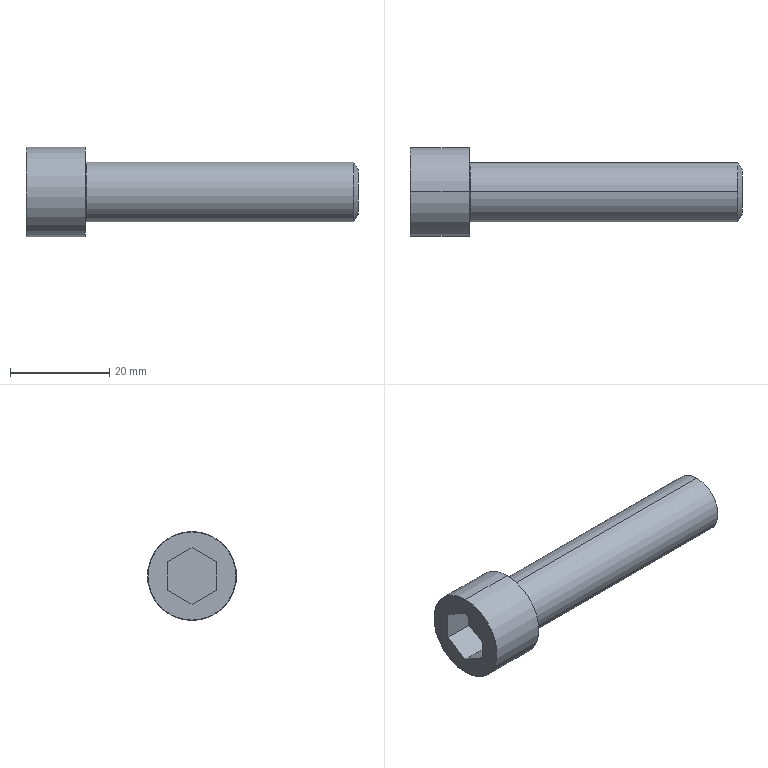Part | SolidWorks | features BaseBody 1 | 1 solid | 20 faces | box 67 x 18 x 18 mm | volume 8742 mm3 | plane 10 | torus 4 | cylinder 4 | cone 2 | commonest cylinder face diameters 12 x2 18 x2
STEP:
#1=CARTESIAN_POINT('',(0.,0.,8.9));
#2=VERTEX_POINT('',#1);
#3=CARTESIAN_POINT('',(0.1,0.,9.));
#4=VERTEX_POINT('',#3);
#5=CARTESIAN_POINT('',(0.1,0.,8.9));
#6=DIRECTION('',(0.,1.,0.));
#7=DIRECTION('',(0.,0.,1.));
#8=AXIS2_PLACEMENT_3D('',#5,#6,#7);
#9=CIRCLE('',#8,0.1);
#10=EDGE_CURVE('',#2,#4,#9,.T.);
#11=ORIENTED_EDGE('',*,*,#10,.F.);
#12=CARTESIAN_POINT('',(0.,0.,-8.9));
#13=VERTEX_POINT('',#12);
#14=CARTESIAN_POINT('',(0.,0.,0.));
#15=DIRECTION('',(-1.,0.,0.));
#16=DIRECTION('',(0.,0.,-1.));
#17=AXIS2_PLACEMENT_3D('',#14,#15,#16);
#18=CIRCLE('',#17,8.9);
#19=EDGE_CURVE('',#13,#2,#18,.T.);
#20=ORIENTED_EDGE('',*,*,#19,.F.);
#21=CARTESIAN_POINT('',(0.1,0.,-9.));
#22=VERTEX_POINT('',#21);
#23=CARTESIAN_POINT('',(0.1,0.,-8.9));
#24=DIRECTION('',(0.,-1.,0.));
#25=DIRECTION('',(0.,0.,-1.));
#26=AXIS2_PLACEMENT_3D('',#23,#24,#25);
#27=CIRCLE('',#26,0.1);
#28=EDGE_CURVE('',#13,#22,#27,.T.);
#29=ORIENTED_EDGE('',*,*,#28,.T.);
#30=CARTESIAN_POINT('',(0.1,0.,0.));
#31=DIRECTION('',(1.,0.,0.));
#32=DIRECTION('',(0.,0.,-1.));
#33=AXIS2_PLACEMENT_3D('',#30,#31,#32);
#34=CIRCLE('',#33,9.);
#35=EDGE_CURVE('',#4,#22,#34,.T.);
#36=ORIENTED_EDGE('',*,*,#35,.F.);
#37=EDGE_LOOP('',(#11,#20,#29,#36));
#38=FACE_OUTER_BOUND('',#37,.T.);
#39=CARTESIAN_POINT('',(0.1,0.,0.));
#40=DIRECTION('',(1.,0.,0.));
#41=DIRECTION('',(0.,0.,-1.));
#42=AXIS2_PLACEMENT_3D('',#39,#40,#41);
#43=TOROIDAL_SURFACE('',#42,8.9,0.1);
#44=ADVANCED_FACE('',(#38),#43,.T.);
#45=CARTESIAN_POINT('',(67.,0.,4.484));
#46=VERTEX_POINT('',#45);
#47=CARTESIAN_POINT('',(67.,0.,-4.484));
#48=VERTEX_POINT('',#47);
#49=CARTESIAN_POINT('',(67.,0.,0.));
#50=DIRECTION('',(-1.,0.,0.));
#51=DIRECTION('',(0.,0.,1.));
#52=AXIS2_PLACEMENT_3D('',#49,#50,#51);
#53=CIRCLE('',#52,4.484);
#54=EDGE_CURVE('',#46,#48,#53,.T.);
#55=ORIENTED_EDGE('',*,*,#54,.F.);
#56=CARTESIAN_POINT('',(67.,0.,0.));
#57=DIRECTION('',(-1.,0.,0.));
#58=DIRECTION('',(0.,0.,1.));
#59=AXIS2_PLACEMENT_3D('',#56,#57,#58);
#60=CIRCLE('',#59,4.484);
#61=EDGE_CURVE('',#48,#46,#60,.T.);
#62=ORIENTED_EDGE('',*,*,#61,.F.);
#63=EDGE_LOOP('',(#55,#62));
#64=FACE_OUTER_BOUND('',#63,.T.);
#65=CARTESIAN_POINT('',(67.,6.,0.));
#66=DIRECTION('',(-1.,0.,0.));
#67=DIRECTION('',(0.,0.,1.));
#68=AXIS2_PLACEMENT_3D('',#65,#66,#67);
#69=PLANE('',#68);
#70=ADVANCED_FACE('',(#64),#69,.F.);
#71=CARTESIAN_POINT('',(66.125,0.,-6.));
#72=VERTEX_POINT('',#71);
#73=CARTESIAN_POINT('',(66.125,0.,-6.));
#74=DIRECTION('',(-0.5,0.,-0.866));
#75=VECTOR('',#74,1000.);
#76=LINE('',#73,#75);
#77=EDGE_CURVE('',#48,#72,#76,.T.);
#78=ORIENTED_EDGE('',*,*,#77,.F.);
#79=ORIENTED_EDGE('',*,*,#61,.T.);
#80=CARTESIAN_POINT('',(66.125,0.,6.));
#81=VERTEX_POINT('',#80);
#82=CARTESIAN_POINT('',(66.125,0.,6.));
#83=DIRECTION('',(-0.5,0.,0.866));
#84=VECTOR('',#83,1000.);
#85=LINE('',#82,#84);
#86=EDGE_CURVE('',#46,#81,#85,.T.);
#87=ORIENTED_EDGE('',*,*,#86,.T.);
#88=CARTESIAN_POINT('',(66.125,0.,0.));
#89=DIRECTION('',(-1.,0.,0.));
#90=DIRECTION('',(0.,0.,1.));
#91=AXIS2_PLACEMENT_3D('',#88,#89,#90);
#92=CIRCLE('',#91,6.);
#93=EDGE_CURVE('',#72,#81,#92,.T.);
#94=ORIENTED_EDGE('',*,*,#93,.F.);
#95=EDGE_LOOP('',(#78,#79,#87,#94));
#96=FACE_OUTER_BOUND('',#95,.T.);
#97=CARTESIAN_POINT('',(66.125,0.,0.));
#98=DIRECTION('',(-1.,0.,0.));
#99=DIRECTION('',(0.,0.,1.));
#100=AXIS2_PLACEMENT_3D('',#97,#98,#99);
#101=CONICAL_SURFACE('',#100,6.,1.047);
#102=ADVANCED_FACE('',(#96),#101,.T.);
#103=CARTESIAN_POINT('',(6.,-4.949,2.857));
#104=VERTEX_POINT('',#103);
#105=CARTESIAN_POINT('',(6.,0.,5.715));
#106=VERTEX_POINT('',#105);
#107=CARTESIAN_POINT('',(6.,-4.949,2.857));
#108=DIRECTION('',(0.,0.866,0.5));
#109=VECTOR('',#108,1000.);
#110=LINE('',#107,#109);
#111=EDGE_CURVE('',#104,#106,#110,.T.);
#112=ORIENTED_EDGE('',*,*,#111,.T.);
#113=CARTESIAN_POINT('',(6.,4.949,2.857));
#114=VERTEX_POINT('',#113);
#115=CARTESIAN_POINT('',(6.,0.,5.715));
#116=DIRECTION('',(0.,0.866,-0.5));
#117=VECTOR('',#116,1000.);
#118=LINE('',#115,#117);
#119=EDGE_CURVE('',#106,#114,#118,.T.);
#120=ORIENTED_EDGE('',*,*,#119,.T.);
#121=CARTESIAN_POINT('',(6.,4.949,-2.857));
#122=VERTEX_POINT('',#121);
#123=CARTESIAN_POINT('',(6.,4.949,2.857));
#124=DIRECTION('',(0.,0.,-1.));
#125=VECTOR('',#124,1000.);
#126=LINE('',#123,#125);
#127=EDGE_CURVE('',#114,#122,#126,.T.);
#128=ORIENTED_EDGE('',*,*,#127,.T.);
#129=CARTESIAN_POINT('',(6.,0.,-5.715));
#130=VERTEX_POINT('',#129);
#131=CARTESIAN_POINT('',(6.,4.949,-2.857));
#132=DIRECTION('',(0.,-0.866,-0.5));
#133=VECTOR('',#132,1000.);
#134=LINE('',#131,#133);
#135=EDGE_CURVE('',#122,#130,#134,.T.);
#136=ORIENTED_EDGE('',*,*,#135,.T.);
#137=CARTESIAN_POINT('',(6.,-4.949,-2.857));
#138=VERTEX_POINT('',#137);
#139=CARTESIAN_POINT('',(6.,0.,-5.715));
#140=DIRECTION('',(0.,-0.866,0.5));
#141=VECTOR('',#140,1000.);
#142=LINE('',#139,#141);
#143=EDGE_CURVE('',#130,#138,#142,.T.);
#144=ORIENTED_EDGE('',*,*,#143,.T.);
#145=CARTESIAN_POINT('',(6.,-4.949,-2.857));
#146=DIRECTION('',(0.,0.,1.));
#147=VECTOR('',#146,1000.);
#148=LINE('',#145,#147);
#149=EDGE_CURVE('',#138,#104,#148,.T.);
#150=ORIENTED_EDGE('',*,*,#149,.T.);
#151=EDGE_LOOP('',(#112,#120,#128,#136,#144,#150));
#152=FACE_OUTER_BOUND('',#151,.T.);
#153=CARTESIAN_POINT('',(6.,-4.949,2.857));
#154=DIRECTION('',(1.,0.,0.));
#155=DIRECTION('',(0.,1.,0.));
#156=AXIS2_PLACEMENT_3D('',#153,#154,#155);
#157=PLANE('',#156);
#158=ADVANCED_FACE('',(#152),#157,.F.);
#159=CARTESIAN_POINT('',(0.,0.,5.715));
#160=VERTEX_POINT('',#159);
#161=CARTESIAN_POINT('',(0.,4.949,2.857));
#162=VERTEX_POINT('',#161);
#163=CARTESIAN_POINT('',(0.,0.,5.715));
#164=DIRECTION('',(0.,0.866,-0.5));
#165=VECTOR('',#164,1000.);
#166=LINE('',#163,#165);
#167=EDGE_CURVE('',#160,#162,#166,.T.);
#168=ORIENTED_EDGE('',*,*,#167,.T.);
#169=CARTESIAN_POINT('',(6.,4.949,2.857));
#170=DIRECTION('',(-1.,0.,0.));
#171=VECTOR('',#170,1000.);
#172=LINE('',#169,#171);
#173=EDGE_CURVE('',#114,#162,#172,.T.);
#174=ORIENTED_EDGE('',*,*,#173,.F.);
#175=ORIENTED_EDGE('',*,*,#119,.F.);
#176=CARTESIAN_POINT('',(6.,0.,5.715));
#177=DIRECTION('',(-1.,0.,0.));
#178=VECTOR('',#177,1000.);
#179=LINE('',#176,#178);
#180=EDGE_CURVE('',#106,#160,#179,.T.);
#181=ORIENTED_EDGE('',*,*,#180,.T.);
#182=EDGE_LOOP('',(#168,#174,#175,#181));
#183=FACE_OUTER_BOUND('',#182,.T.);
#184=CARTESIAN_POINT('',(6.,0.,5.715));
#185=DIRECTION('',(0.,0.5,0.866));
#186=DIRECTION('',(1.,0.,0.));
#187=AXIS2_PLACEMENT_3D('',#184,#185,#186);
#188=PLANE('',#187);
#189=ADVANCED_FACE('',(#183),#188,.F.);
#190=CARTESIAN_POINT('',(0.,4.949,-2.857));
#191=VERTEX_POINT('',#190);
#192=CARTESIAN_POINT('',(0.,4.949,2.857));
#193=DIRECTION('',(0.,0.,-1.));
#194=VECTOR('',#193,1000.);
#195=LINE('',#192,#194);
#196=EDGE_CURVE('',#162,#191,#195,.T.);
#197=ORIENTED_EDGE('',*,*,#196,.T.);
#198=CARTESIAN_POINT('',(6.,4.949,-2.857));
#199=DIRECTION('',(-1.,0.,0.));
#200=VECTOR('',#199,1000.);
#201=LINE('',#198,#200);
#202=EDGE_CURVE('',#122,#191,#201,.T.);
#203=ORIENTED_EDGE('',*,*,#202,.F.);
#204=ORIENTED_EDGE('',*,*,#127,.F.);
#205=ORIENTED_EDGE('',*,*,#173,.T.);
#206=EDGE_LOOP('',(#197,#203,#204,#205));
#207=FACE_OUTER_BOUND('',#206,.T.);
#208=CARTESIAN_POINT('',(6.,4.949,2.857));
#209=DIRECTION('',(0.,1.,0.));
#210=DIRECTION('',(0.,0.,-1.));
#211=AXIS2_PLACEMENT_3D('',#208,#209,#210);
#212=PLANE('',#211);
#213=ADVANCED_FACE('',(#207),#212,.F.);
#214=CARTESIAN_POINT('',(0.,0.,-5.715));
#215=VERTEX_POINT('',#214);
#216=CARTESIAN_POINT('',(0.,4.949,-2.857));
#217=DIRECTION('',(0.,-0.866,-0.5));
#218=VECTOR('',#217,1000.);
#219=LINE('',#216,#218);
#220=EDGE_CURVE('',#191,#215,#219,.T.);
#221=ORIENTED_EDGE('',*,*,#220,.T.);
#222=CARTESIAN_POINT('',(6.,0.,-5.715));
#223=DIRECTION('',(-1.,0.,0.));
#224=VECTOR('',#223,1000.);
#225=LINE('',#222,#224);
#226=EDGE_CURVE('',#130,#215,#225,.T.);
#227=ORIENTED_EDGE('',*,*,#226,.F.);
#228=ORIENTED_EDGE('',*,*,#135,.F.);
#229=ORIENTED_EDGE('',*,*,#202,.T.);
#230=EDGE_LOOP('',(#221,#227,#228,#229));
#231=FACE_OUTER_BOUND('',#230,.T.);
#232=CARTESIAN_POINT('',(6.,4.949,-2.857));
#233=DIRECTION('',(0.,0.5,-0.866));
#234=DIRECTION('',(-1.,0.,0.));
#235=AXIS2_PLACEMENT_3D('',#232,#233,#234);
#236=PLANE('',#235);
#237=ADVANCED_FACE('',(#231),#236,.F.);
#238=CARTESIAN_POINT('',(0.,-4.949,-2.857));
#239=VERTEX_POINT('',#238);
#240=CARTESIAN_POINT('',(0.,0.,-5.715));
#241=DIRECTION('',(0.,-0.866,0.5));
#242=VECTOR('',#241,1000.);
#243=LINE('',#240,#242);
#244=EDGE_CURVE('',#215,#239,#243,.T.);
#245=ORIENTED_EDGE('',*,*,#244,.T.);
#246=CARTESIAN_POINT('',(6.,-4.949,-2.857));
#247=DIRECTION('',(-1.,0.,0.));
#248=VECTOR('',#247,1000.);
#249=LINE('',#246,#248);
#250=EDGE_CURVE('',#138,#239,#249,.T.);
#251=ORIENTED_EDGE('',*,*,#250,.F.);
#252=ORIENTED_EDGE('',*,*,#143,.F.);
#253=ORIENTED_EDGE('',*,*,#226,.T.);
#254=EDGE_LOOP('',(#245,#251,#252,#253));
#255=FACE_OUTER_BOUND('',#254,.T.);
#256=CARTESIAN_POINT('',(6.,0.,-5.715));
#257=DIRECTION('',(0.,-0.5,-0.866));
#258=DIRECTION('',(0.,-0.866,0.5));
#259=AXIS2_PLACEMENT_3D('',#256,#257,#258);
#260=PLANE('',#259);
#261=ADVANCED_FACE('',(#255),#260,.F.);
#262=CARTESIAN_POINT('',(0.,-4.949,2.857));
#263=VERTEX_POINT('',#262);
#264=CARTESIAN_POINT('',(0.,-4.949,-2.857));
#265=DIRECTION('',(0.,0.,1.));
#266=VECTOR('',#265,1000.);
#267=LINE('',#264,#266);
#268=EDGE_CURVE('',#239,#263,#267,.T.);
#269=ORIENTED_EDGE('',*,*,#268,.T.);
#270=CARTESIAN_POINT('',(6.,-4.949,2.857));
#271=DIRECTION('',(-1.,0.,0.));
#272=VECTOR('',#271,1000.);
#273=LINE('',#270,#272);
#274=EDGE_CURVE('',#104,#263,#273,.T.);
#275=ORIENTED_EDGE('',*,*,#274,.F.);
#276=ORIENTED_EDGE('',*,*,#149,.F.);
#277=ORIENTED_EDGE('',*,*,#250,.T.);
#278=EDGE_LOOP('',(#269,#275,#276,#277));
#279=FACE_OUTER_BOUND('',#278,.T.);
#280=CARTESIAN_POINT('',(6.,-4.949,-2.857));
#281=DIRECTION('',(0.,-1.,0.));
#282=DIRECTION('',(0.,0.,-1.));
#283=AXIS2_PLACEMENT_3D('',#280,#281,#282);
#284=PLANE('',#283);
#285=ADVANCED_FACE('',(#279),#284,.F.);
#286=CARTESIAN_POINT('',(0.,-4.949,2.857));
#287=DIRECTION('',(0.,0.866,0.5));
#288=VECTOR('',#287,1000.);
#289=LINE('',#286,#288);
#290=EDGE_CURVE('',#263,#160,#289,.T.);
#291=ORIENTED_EDGE('',*,*,#290,.T.);
#292=ORIENTED_EDGE('',*,*,#180,.F.);
#293=ORIENTED_EDGE('',*,*,#111,.F.);
#294=ORIENTED_EDGE('',*,*,#274,.T.);
#295=EDGE_LOOP('',(#291,#292,#293,#294));
#296=FACE_OUTER_BOUND('',#295,.T.);
#297=CARTESIAN_POINT('',(6.,-4.949,2.857));
#298=DIRECTION('',(0.,-0.5,0.866));
#299=DIRECTION('',(-1.,0.,0.));
#300=AXIS2_PLACEMENT_3D('',#297,#298,#299);
#301=PLANE('',#300);
#302=ADVANCED_FACE('',(#296),#301,.F.);
#303=CARTESIAN_POINT('',(12.,0.,-6.2));
#304=VERTEX_POINT('',#303);
#305=CARTESIAN_POINT('',(12.2,0.,-6.));
#306=VERTEX_POINT('',#305);
#307=CARTESIAN_POINT('',(12.2,0.,-6.2));
#308=DIRECTION('',(0.,1.,0.));
#309=DIRECTION('',(0.,0.,1.));
#310=AXIS2_PLACEMENT_3D('',#307,#308,#309);
#311=CIRCLE('',#310,0.2);
#312=EDGE_CURVE('',#304,#306,#311,.T.);
#313=ORIENTED_EDGE('',*,*,#312,.F.);
#314=CARTESIAN_POINT('',(12.,0.,6.2));
#315=VERTEX_POINT('',#314);
#316=CARTESIAN_POINT('',(12.,0.,0.));
#317=DIRECTION('',(-1.,0.,0.));
#318=DIRECTION('',(0.,0.,1.));
#319=AXIS2_PLACEMENT_3D('',#316,#317,#318);
#320=CIRCLE('',#319,6.2);
#321=EDGE_CURVE('',#315,#304,#320,.T.);
#322=ORIENTED_EDGE('',*,*,#321,.F.);
#323=CARTESIAN_POINT('',(12.2,0.,6.));
#324=VERTEX_POINT('',#323);
#325=CARTESIAN_POINT('',(12.2,0.,6.2));
#326=DIRECTION('',(0.,-1.,0.));
#327=DIRECTION('',(0.,0.,-1.));
#328=AXIS2_PLACEMENT_3D('',#325,#326,#327);
#329=CIRCLE('',#328,0.2);
#330=EDGE_CURVE('',#315,#324,#329,.T.);
#331=ORIENTED_EDGE('',*,*,#330,.T.);
#332=CARTESIAN_POINT('',(12.2,0.,0.));
#333=DIRECTION('',(-1.,0.,0.));
#334=DIRECTION('',(0.,0.,1.));
#335=AXIS2_PLACEMENT_3D('',#332,#333,#334);
#336=CIRCLE('',#335,6.);
#337=EDGE_CURVE('',#324,#306,#336,.T.);
#338=ORIENTED_EDGE('',*,*,#337,.T.);
#339=EDGE_LOOP('',(#313,#322,#331,#338));
#340=FACE_OUTER_BOUND('',#339,.T.);
#341=CARTESIAN_POINT('',(12.2,0.,0.));
#342=DIRECTION('',(-1.,0.,0.));
#343=DIRECTION('',(0.,0.,1.));
#344=AXIS2_PLACEMENT_3D('',#341,#342,#343);
#345=TOROIDAL_SURFACE('',#344,6.2,0.2);
#346=ADVANCED_FACE('',(#340),#345,.F.);
#347=ORIENTED_EDGE('',*,*,#321,.T.);
#348=CARTESIAN_POINT('',(12.,0.,0.));
#349=DIRECTION('',(-1.,0.,0.));
#350=DIRECTION('',(0.,0.,1.));
#351=AXIS2_PLACEMENT_3D('',#348,#349,#350);
#352=CIRCLE('',#351,6.2);
#353=EDGE_CURVE('',#304,#315,#352,.T.);
#354=ORIENTED_EDGE('',*,*,#353,.T.);
#355=EDGE_LOOP('',(#347,#354));
#356=FACE_BOUND('',#355,.T.);
#357=CARTESIAN_POINT('',(12.,0.,9.));
#358=VERTEX_POINT('',#357);
#359=CARTESIAN_POINT('',(12.,0.,-9.));
#360=VERTEX_POINT('',#359);
#361=CARTESIAN_POINT('',(12.,0.,0.));
#362=DIRECTION('',(-1.,0.,0.));
#363=DIRECTION('',(0.,0.,1.));
#364=AXIS2_PLACEMENT_3D('',#361,#362,#363);
#365=CIRCLE('',#364,9.);
#366=EDGE_CURVE('',#358,#360,#365,.T.);
#367=ORIENTED_EDGE('',*,*,#366,.F.);
#368=CARTESIAN_POINT('',(12.,0.,0.));
#369=DIRECTION('',(-1.,0.,0.));
#370=DIRECTION('',(0.,0.,1.));
#371=AXIS2_PLACEMENT_3D('',#368,#369,#370);
#372=CIRCLE('',#371,9.);
#373=EDGE_CURVE('',#360,#358,#372,.T.);
#374=ORIENTED_EDGE('',*,*,#373,.F.);
#375=EDGE_LOOP('',(#367,#374));
#376=FACE_OUTER_BOUND('',#375,.T.);
#377=CARTESIAN_POINT('',(12.,9.,0.));
#378=DIRECTION('',(-1.,0.,0.));
#379=DIRECTION('',(0.,0.,1.));
#380=AXIS2_PLACEMENT_3D('',#377,#378,#379);
#381=PLANE('',#380);
#382=ADVANCED_FACE('',(#356,#376),#381,.F.);
#383=CARTESIAN_POINT('',(0.,0.,-9.));
#384=DIRECTION('',(-1.,0.,0.));
#385=VECTOR('',#384,1000.);
#386=LINE('',#383,#385);
#387=EDGE_CURVE('',#360,#22,#386,.T.);
#388=ORIENTED_EDGE('',*,*,#387,.F.);
#389=ORIENTED_EDGE('',*,*,#373,.T.);
#390=CARTESIAN_POINT('',(0.,0.,9.));
#391=DIRECTION('',(-1.,0.,0.));
#392=VECTOR('',#391,1000.);
#393=LINE('',#390,#392);
#394=EDGE_CURVE('',#358,#4,#393,.T.);
#395=ORIENTED_EDGE('',*,*,#394,.T.);
#396=ORIENTED_EDGE('',*,*,#35,.T.);
#397=EDGE_LOOP('',(#388,#389,#395,#396));
#398=FACE_OUTER_BOUND('',#397,.T.);
#399=CARTESIAN_POINT('',(0.,0.,0.));
#400=DIRECTION('',(-1.,0.,0.));
#401=DIRECTION('',(0.,0.,1.));
#402=AXIS2_PLACEMENT_3D('',#399,#400,#401);
#403=CYLINDRICAL_SURFACE('',#402,9.);
#404=ADVANCED_FACE('',(#398),#403,.T.);
#405=ORIENTED_EDGE('',*,*,#167,.F.);
#406=ORIENTED_EDGE('',*,*,#290,.F.);
#407=ORIENTED_EDGE('',*,*,#268,.F.);
#408=ORIENTED_EDGE('',*,*,#244,.F.);
#409=ORIENTED_EDGE('',*,*,#220,.F.);
#410=ORIENTED_EDGE('',*,*,#196,.F.);
#411=EDGE_LOOP('',(#405,#406,#407,#408,#409,#410));
#412=FACE_BOUND('',#411,.T.);
#413=ORIENTED_EDGE('',*,*,#19,.T.);
#414=CARTESIAN_POINT('',(0.,0.,0.));
#415=DIRECTION('',(-1.,0.,0.));
#416=DIRECTION('',(0.,0.,-1.));
#417=AXIS2_PLACEMENT_3D('',#414,#415,#416);
#418=CIRCLE('',#417,8.9);
#419=EDGE_CURVE('',#2,#13,#418,.T.);
#420=ORIENTED_EDGE('',*,*,#419,.T.);
#421=EDGE_LOOP('',(#413,#420));
#422=FACE_OUTER_BOUND('',#421,.T.);
#423=CARTESIAN_POINT('',(0.,0.,0.));
#424=DIRECTION('',(1.,0.,0.));
#425=DIRECTION('',(0.,1.,0.));
#426=AXIS2_PLACEMENT_3D('',#423,#424,#425);
#427=PLANE('',#426);
#428=ADVANCED_FACE('',(#412,#422),#427,.F.);
#429=CARTESIAN_POINT('',(0.,0.,-6.));
#430=DIRECTION('',(-1.,0.,0.));
#431=VECTOR('',#430,1000.);
#432=LINE('',#429,#431);
#433=EDGE_CURVE('',#72,#306,#432,.T.);
#434=ORIENTED_EDGE('',*,*,#433,.F.);
#435=ORIENTED_EDGE('',*,*,#93,.T.);
#436=CARTESIAN_POINT('',(0.,0.,6.));
#437=DIRECTION('',(-1.,0.,0.));
#438=VECTOR('',#437,1000.);
#439=LINE('',#436,#438);
#440=EDGE_CURVE('',#81,#324,#439,.T.);
#441=ORIENTED_EDGE('',*,*,#440,.T.);
#442=CARTESIAN_POINT('',(12.2,0.,0.));
#443=DIRECTION('',(-1.,0.,0.));
#444=DIRECTION('',(0.,0.,1.));
#445=AXIS2_PLACEMENT_3D('',#442,#443,#444);
#446=CIRCLE('',#445,6.);
#447=EDGE_CURVE('',#306,#324,#446,.T.);
#448=ORIENTED_EDGE('',*,*,#447,.F.);
#449=EDGE_LOOP('',(#434,#435,#441,#448));
#450=FACE_OUTER_BOUND('',#449,.T.);
#451=CARTESIAN_POINT('',(0.,0.,0.));
#452=DIRECTION('',(-1.,0.,0.));
#453=DIRECTION('',(0.,0.,1.));
#454=AXIS2_PLACEMENT_3D('',#451,#452,#453);
#455=CYLINDRICAL_SURFACE('',#454,6.);
#456=ADVANCED_FACE('',(#450),#455,.T.);
#457=CARTESIAN_POINT('',(66.125,0.,0.));
#458=DIRECTION('',(-1.,0.,0.));
#459=DIRECTION('',(0.,0.,1.));
#460=AXIS2_PLACEMENT_3D('',#457,#458,#459);
#461=CIRCLE('',#460,6.);
#462=EDGE_CURVE('',#81,#72,#461,.T.);
#463=ORIENTED_EDGE('',*,*,#462,.T.);
#464=ORIENTED_EDGE('',*,*,#433,.T.);
#465=ORIENTED_EDGE('',*,*,#337,.F.);
#466=ORIENTED_EDGE('',*,*,#440,.F.);
#467=EDGE_LOOP('',(#463,#464,#465,#466));
#468=FACE_OUTER_BOUND('',#467,.T.);
#469=CARTESIAN_POINT('',(0.,0.,0.));
#470=DIRECTION('',(-1.,0.,0.));
#471=DIRECTION('',(0.,0.,1.));
#472=AXIS2_PLACEMENT_3D('',#469,#470,#471);
#473=CYLINDRICAL_SURFACE('',#472,6.);
#474=ADVANCED_FACE('',(#468),#473,.T.);
#475=ORIENTED_EDGE('',*,*,#366,.T.);
#476=ORIENTED_EDGE('',*,*,#387,.T.);
#477=CARTESIAN_POINT('',(0.1,0.,0.));
#478=DIRECTION('',(1.,0.,0.));
#479=DIRECTION('',(0.,0.,-1.));
#480=AXIS2_PLACEMENT_3D('',#477,#478,#479);
#481=CIRCLE('',#480,9.);
#482=EDGE_CURVE('',#22,#4,#481,.T.);
#483=ORIENTED_EDGE('',*,*,#482,.T.);
#484=ORIENTED_EDGE('',*,*,#394,.F.);
#485=EDGE_LOOP('',(#475,#476,#483,#484));
#486=FACE_OUTER_BOUND('',#485,.T.);
#487=CARTESIAN_POINT('',(0.,0.,0.));
#488=DIRECTION('',(-1.,0.,0.));
#489=DIRECTION('',(0.,0.,1.));
#490=AXIS2_PLACEMENT_3D('',#487,#488,#489);
#491=CYLINDRICAL_SURFACE('',#490,9.);
#492=ADVANCED_FACE('',(#486),#491,.T.);
#493=ORIENTED_EDGE('',*,*,#353,.F.);
#494=ORIENTED_EDGE('',*,*,#312,.T.);
#495=ORIENTED_EDGE('',*,*,#447,.T.);
#496=ORIENTED_EDGE('',*,*,#330,.F.);
#497=EDGE_LOOP('',(#493,#494,#495,#496));
#498=FACE_OUTER_BOUND('',#497,.T.);
#499=CARTESIAN_POINT('',(12.2,0.,0.));
#500=DIRECTION('',(-1.,0.,0.));
#501=DIRECTION('',(0.,0.,1.));
#502=AXIS2_PLACEMENT_3D('',#499,#500,#501);
#503=TOROIDAL_SURFACE('',#502,6.2,0.2);
#504=ADVANCED_FACE('',(#498),#503,.F.);
#505=ORIENTED_EDGE('',*,*,#54,.T.);
#506=ORIENTED_EDGE('',*,*,#77,.T.);
#507=ORIENTED_EDGE('',*,*,#462,.F.);
#508=ORIENTED_EDGE('',*,*,#86,.F.);
#509=EDGE_LOOP('',(#505,#506,#507,#508));
#510=FACE_OUTER_BOUND('',#509,.T.);
#511=CARTESIAN_POINT('',(66.125,0.,0.));
#512=DIRECTION('',(-1.,0.,0.));
#513=DIRECTION('',(0.,0.,1.));
#514=AXIS2_PLACEMENT_3D('',#511,#512,#513);
#515=CONICAL_SURFACE('',#514,6.,1.047);
#516=ADVANCED_FACE('',(#510),#515,.T.);
#517=ORIENTED_EDGE('',*,*,#419,.F.);
#518=ORIENTED_EDGE('',*,*,#10,.T.);
#519=ORIENTED_EDGE('',*,*,#482,.F.);
#520=ORIENTED_EDGE('',*,*,#28,.F.);
#521=EDGE_LOOP('',(#517,#518,#519,#520));
#522=FACE_OUTER_BOUND('',#521,.T.);
#523=CARTESIAN_POINT('',(0.1,0.,0.));
#524=DIRECTION('',(1.,0.,0.));
#525=DIRECTION('',(0.,0.,-1.));
#526=AXIS2_PLACEMENT_3D('',#523,#524,#525);
#527=TOROIDAL_SURFACE('',#526,8.9,0.1);
#528=ADVANCED_FACE('',(#522),#527,.T.);
#529=CLOSED_SHELL('',(#44,#70,#102,#158,#189,#213,#237,#261,#285,#302,#346,#382,#404,#428,#456,#474,#492,#504,#516,#528));
#530=MANIFOLD_SOLID_BREP('',#529);
#531=CARTESIAN_POINT('',(0.,0.,0.));
#532=DIRECTION('',(0.,0.,1.));
#533=DIRECTION('',(1.,0.,0.));
#534=AXIS2_PLACEMENT_3D('',#531,#532,#533);
#535=(LENGTH_UNIT()NAMED_UNIT(*)SI_UNIT(.MILLI.,.METRE.));
#536=UNCERTAINTY_MEASURE_WITH_UNIT(LENGTH_MEASURE(0.00001),#535,'','');
#537=(NAMED_UNIT(*)PLANE_ANGLE_UNIT()SI_UNIT($,.RADIAN.));
#538=(NAMED_UNIT(*)SI_UNIT($,.STERADIAN.)SOLID_ANGLE_UNIT());
#539=(GEOMETRIC_REPRESENTATION_CONTEXT(3)GLOBAL_UNCERTAINTY_ASSIGNED_CONTEXT((#536))GLOBAL_UNIT_ASSIGNED_CONTEXT((#535,#537,#538))REPRESENTATION_CONTEXT('',''));
#540=ADVANCED_BREP_SHAPE_REPRESENTATION('',(#530,#534),#539);